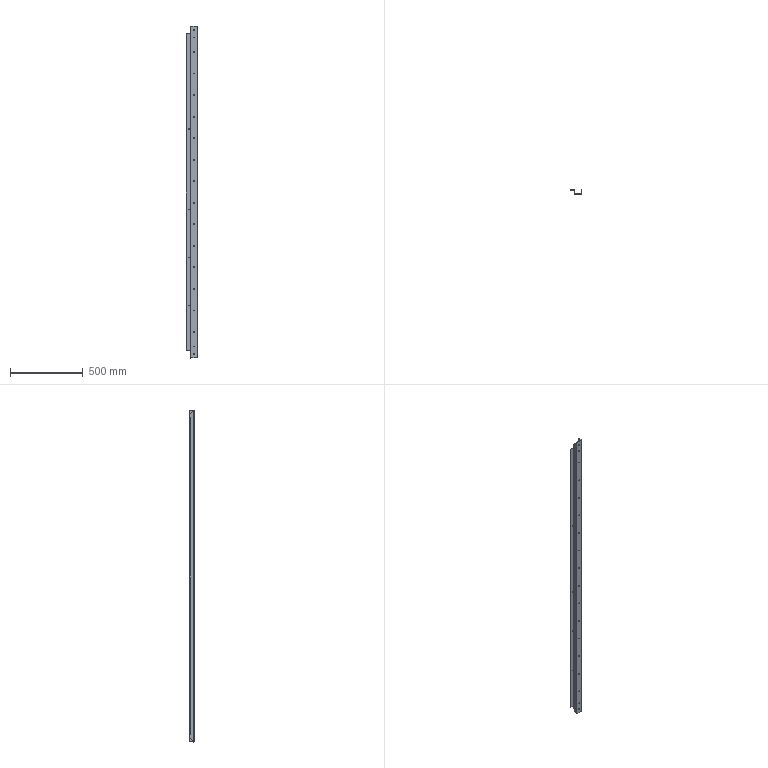Part | STEP file | SX-004-07 | 1 solid | 104 faces | box 78 x 30 x 2285 mm | volume 595601 mm3 | cylinder 58 | plane 44 | spline 2 | commonest cylinder face diameters 6 x32 8 x16 3 x4 0.4 x3 4.4 x3